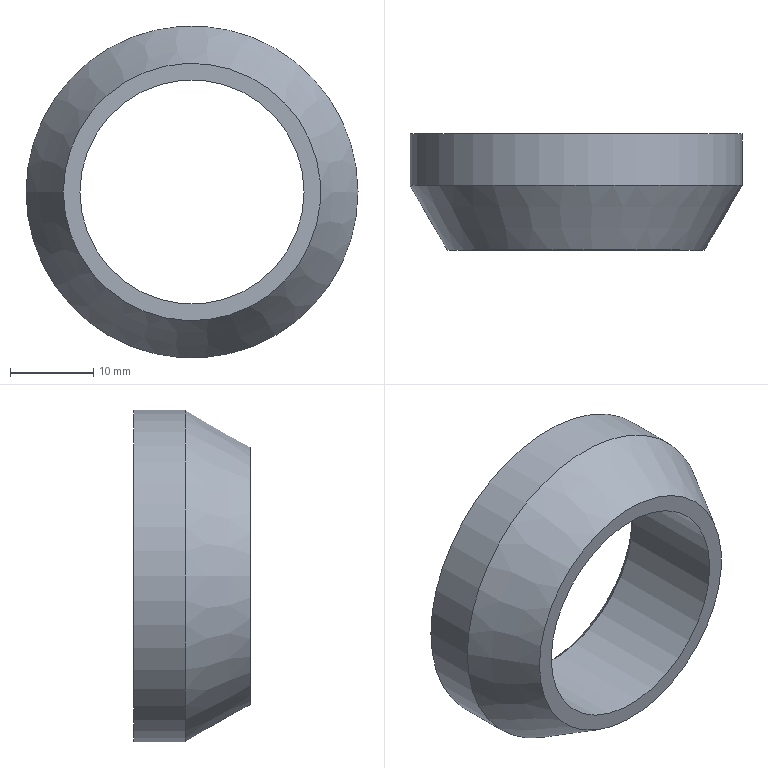Part | NX | features solid 2 | 1 solid | 6 faces | box 40 x 14 x 40 mm | volume 7511 mm3 | plane 2 | cylinder 2 | cone 2 | commonest cylinder face diameters 27 x1 40 x1
STEP:
#1=CARTESIAN_POINT('',(770.7,365.,148.5));
#2=VERTEX_POINT('',#1);
#3=CARTESIAN_POINT('',(785.,365.,148.5));
#4=DIRECTION('',(0.,-1.,0.));
#5=DIRECTION('',(-1.,0.,0.));
#6=AXIS2_PLACEMENT_3D('',#3,#4,#5);
#7=CIRCLE('',#6,14.3);
#8=EDGE_CURVE('',#2,#2,#7,.F.);
#9=ORIENTED_EDGE('',*,*,#8,.F.);
#10=EDGE_LOOP('',(#9));
#11=FACE_BOUND('',#10,.T.);
#12=CARTESIAN_POINT('',(765.,365.,148.5));
#13=VERTEX_POINT('',#12);
#14=CARTESIAN_POINT('',(785.,365.,148.5));
#15=DIRECTION('',(0.,-1.,0.));
#16=DIRECTION('',(-1.,0.,0.));
#17=AXIS2_PLACEMENT_3D('',#14,#15,#16);
#18=CIRCLE('',#17,20.);
#19=EDGE_CURVE('',#13,#13,#18,.T.);
#20=ORIENTED_EDGE('',*,*,#19,.F.);
#21=EDGE_LOOP('',(#20));
#22=FACE_BOUND('',#21,.T.);
#23=CARTESIAN_POINT('',(785.,365.,135.));
#24=DIRECTION('',(0.,1.,0.));
#25=DIRECTION('',(-1.,0.,0.));
#26=AXIS2_PLACEMENT_3D('',#23,#24,#25);
#27=PLANE('',#26);
#28=ADVANCED_FACE('',(#11,#22),#27,.T.);
#29=CARTESIAN_POINT('',(765.,358.794,148.5));
#30=VERTEX_POINT('',#29);
#31=CARTESIAN_POINT('',(785.,358.794,148.5));
#32=DIRECTION('',(0.,-1.,0.));
#33=DIRECTION('',(-1.,0.,0.));
#34=AXIS2_PLACEMENT_3D('',#31,#32,#33);
#35=CIRCLE('',#34,20.);
#36=EDGE_CURVE('',#30,#30,#35,.T.);
#37=ORIENTED_EDGE('',*,*,#36,.F.);
#38=EDGE_LOOP('',(#37));
#39=FACE_BOUND('',#38,.T.);
#40=ORIENTED_EDGE('',*,*,#19,.T.);
#41=EDGE_LOOP('',(#40));
#42=FACE_BOUND('',#41,.T.);
#43=CARTESIAN_POINT('',(785.,351.,148.5));
#44=DIRECTION('',(0.,1.,0.));
#45=DIRECTION('',(-1.,0.,0.));
#46=AXIS2_PLACEMENT_3D('',#43,#44,#45);
#47=CYLINDRICAL_SURFACE('',#46,20.);
#48=ADVANCED_FACE('',(#39,#42),#47,.T.);
#49=ORIENTED_EDGE('',*,*,#36,.T.);
#50=EDGE_LOOP('',(#49));
#51=FACE_BOUND('',#50,.T.);
#52=CARTESIAN_POINT('',(769.5,351.,148.5));
#53=VERTEX_POINT('',#52);
#54=CARTESIAN_POINT('',(785.,351.,148.5));
#55=DIRECTION('',(0.,-1.,0.));
#56=DIRECTION('',(-1.,0.,0.));
#57=AXIS2_PLACEMENT_3D('',#54,#55,#56);
#58=CIRCLE('',#57,15.5);
#59=EDGE_CURVE('',#53,#53,#58,.T.);
#60=ORIENTED_EDGE('',*,*,#59,.F.);
#61=EDGE_LOOP('',(#60));
#62=FACE_BOUND('',#61,.T.);
#63=CARTESIAN_POINT('',(785.,351.,148.5));
#64=DIRECTION('',(0.,1.,0.));
#65=DIRECTION('',(-1.,0.,0.));
#66=AXIS2_PLACEMENT_3D('',#63,#64,#65);
#67=CONICAL_SURFACE('',#66,15.5,0.5236);
#68=ADVANCED_FACE('',(#51,#62),#67,.T.);
#69=ORIENTED_EDGE('',*,*,#59,.T.);
#70=EDGE_LOOP('',(#69));
#71=FACE_BOUND('',#70,.T.);
#72=CARTESIAN_POINT('',(771.5,351.,148.5));
#73=VERTEX_POINT('',#72);
#74=CARTESIAN_POINT('',(785.,351.,148.5));
#75=DIRECTION('',(0.,-1.,0.));
#76=DIRECTION('',(-1.,0.,0.));
#77=AXIS2_PLACEMENT_3D('',#74,#75,#76);
#78=CIRCLE('',#77,13.5);
#79=EDGE_CURVE('',#73,#73,#78,.T.);
#80=ORIENTED_EDGE('',*,*,#79,.F.);
#81=EDGE_LOOP('',(#80));
#82=FACE_BOUND('',#81,.T.);
#83=CARTESIAN_POINT('',(785.,351.,135.));
#84=DIRECTION('',(0.,1.,0.));
#85=DIRECTION('',(-1.,0.,0.));
#86=AXIS2_PLACEMENT_3D('',#83,#84,#85);
#87=PLANE('',#86);
#88=ADVANCED_FACE('',(#71,#82),#87,.F.);
#89=CARTESIAN_POINT('',(771.5,364.2,148.5));
#90=VERTEX_POINT('',#89);
#91=CARTESIAN_POINT('',(785.,364.2,148.5));
#92=DIRECTION('',(0.,-1.,0.));
#93=DIRECTION('',(-1.,0.,0.));
#94=AXIS2_PLACEMENT_3D('',#91,#92,#93);
#95=CIRCLE('',#94,13.5);
#96=EDGE_CURVE('',#90,#90,#95,.T.);
#97=ORIENTED_EDGE('',*,*,#96,.F.);
#98=EDGE_LOOP('',(#97));
#99=FACE_BOUND('',#98,.T.);
#100=ORIENTED_EDGE('',*,*,#79,.T.);
#101=EDGE_LOOP('',(#100));
#102=FACE_BOUND('',#101,.T.);
#103=CARTESIAN_POINT('',(785.,351.,148.5));
#104=DIRECTION('',(0.,1.,0.));
#105=DIRECTION('',(-1.,0.,0.));
#106=AXIS2_PLACEMENT_3D('',#103,#104,#105);
#107=CYLINDRICAL_SURFACE('',#106,13.5);
#108=ADVANCED_FACE('',(#99,#102),#107,.F.);
#109=ORIENTED_EDGE('',*,*,#8,.T.);
#110=EDGE_LOOP('',(#109));
#111=FACE_BOUND('',#110,.T.);
#112=ORIENTED_EDGE('',*,*,#96,.T.);
#113=EDGE_LOOP('',(#112));
#114=FACE_BOUND('',#113,.T.);
#115=CARTESIAN_POINT('',(785.,364.2,148.5));
#116=DIRECTION('',(0.,1.,0.));
#117=DIRECTION('',(-1.,0.,0.));
#118=AXIS2_PLACEMENT_3D('',#115,#116,#117);
#119=CONICAL_SURFACE('',#118,13.5,0.7854);
#120=ADVANCED_FACE('',(#111,#114),#119,.F.);
#121=CLOSED_SHELL('',(#28,#48,#68,#88,#108,#120));
#122=MANIFOLD_SOLID_BREP('',#121);
#123=(LENGTH_UNIT()NAMED_UNIT(*)SI_UNIT(.MILLI.,.METRE.));
#124=UNCERTAINTY_MEASURE_WITH_UNIT(LENGTH_MEASURE(0.00001),#123,'','');
#125=(NAMED_UNIT(*)PLANE_ANGLE_UNIT()SI_UNIT($,.RADIAN.));
#126=(NAMED_UNIT(*)SI_UNIT($,.STERADIAN.)SOLID_ANGLE_UNIT());
#127=(GEOMETRIC_REPRESENTATION_CONTEXT(3)GLOBAL_UNCERTAINTY_ASSIGNED_CONTEXT((#124))GLOBAL_UNIT_ASSIGNED_CONTEXT((#123,#125,#126))REPRESENTATION_CONTEXT('',''));
#128=ADVANCED_BREP_SHAPE_REPRESENTATION('',(#122),#127);